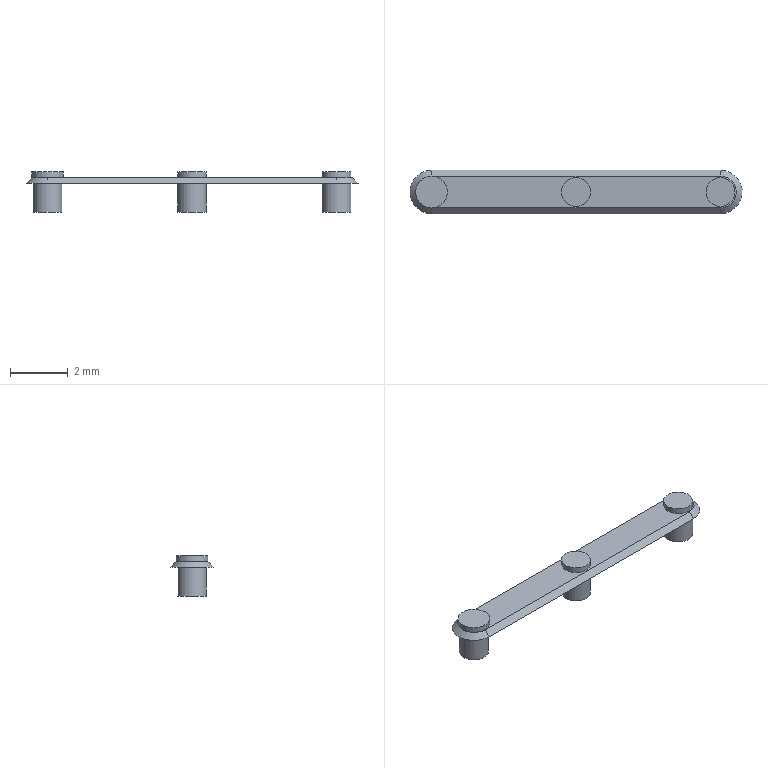Part | NX | features DATUM_CSYS 4, EXTRUDE 3, SKETCH 3, CHAMFER 1 | 7 solids | 24 faces | box 11.5 x 1.5 x 1.4 mm | volume 5.728 mm3 | plane 16 | cylinder 6 | cone 2 | commonest cylinder face diameters 1 x5 1.1 x1
STEP:
#1=CARTESIAN_POINT('',(0.5,0.,1.));
#2=VERTEX_POINT('',#1);
#3=CARTESIAN_POINT('',(0.,0.,1.));
#4=DIRECTION('',(0.,0.,1.));
#5=DIRECTION('',(1.,0.,0.));
#6=AXIS2_PLACEMENT_3D('',#3,#4,#5);
#7=CIRCLE('',#6,0.5);
#8=EDGE_CURVE('',#2,#2,#7,.T.);
#9=ORIENTED_EDGE('',*,*,#8,.F.);
#10=EDGE_LOOP('',(#9));
#11=FACE_BOUND('',#10,.T.);
#12=CARTESIAN_POINT('',(0.5,0.,0.));
#13=VERTEX_POINT('',#12);
#14=CARTESIAN_POINT('',(0.,0.,0.));
#15=DIRECTION('',(0.,0.,1.));
#16=DIRECTION('',(1.,0.,0.));
#17=AXIS2_PLACEMENT_3D('',#14,#15,#16);
#18=CIRCLE('',#17,0.5);
#19=EDGE_CURVE('',#13,#13,#18,.T.);
#20=ORIENTED_EDGE('',*,*,#19,.T.);
#21=EDGE_LOOP('',(#20));
#22=FACE_BOUND('',#21,.T.);
#23=CARTESIAN_POINT('',(0.,0.,1.));
#24=DIRECTION('',(0.,0.,-1.));
#25=DIRECTION('',(-1.,0.,0.));
#26=AXIS2_PLACEMENT_3D('',#23,#24,#25);
#27=CYLINDRICAL_SURFACE('',#26,0.5);
#28=ADVANCED_FACE('',(#11,#22),#27,.T.);
#29=ORIENTED_EDGE('',*,*,#8,.T.);
#30=EDGE_LOOP('',(#29));
#31=FACE_BOUND('',#30,.T.);
#32=CARTESIAN_POINT('',(0.,0.,1.));
#33=DIRECTION('',(0.,0.,1.));
#34=DIRECTION('',(1.,0.,0.));
#35=AXIS2_PLACEMENT_3D('',#32,#33,#34);
#36=PLANE('',#35);
#37=ADVANCED_FACE('',(#31),#36,.T.);
#38=ORIENTED_EDGE('',*,*,#19,.F.);
#39=EDGE_LOOP('',(#38));
#40=FACE_BOUND('',#39,.T.);
#41=CARTESIAN_POINT('',(0.,0.,0.));
#42=DIRECTION('',(0.,0.,1.));
#43=DIRECTION('',(1.,0.,0.));
#44=AXIS2_PLACEMENT_3D('',#41,#42,#43);
#45=PLANE('',#44);
#46=ADVANCED_FACE('',(#40),#45,.F.);
#47=CLOSED_SHELL('',(#28,#37,#46));
#48=MANIFOLD_SOLID_BREP('',#47);
#49=CARTESIAN_POINT('',(5.5,0.,1.));
#50=VERTEX_POINT('',#49);
#51=CARTESIAN_POINT('',(5.,0.,1.));
#52=DIRECTION('',(0.,0.,1.));
#53=DIRECTION('',(1.,0.,0.));
#54=AXIS2_PLACEMENT_3D('',#51,#52,#53);
#55=CIRCLE('',#54,0.5);
#56=EDGE_CURVE('',#50,#50,#55,.T.);
#57=ORIENTED_EDGE('',*,*,#56,.F.);
#58=EDGE_LOOP('',(#57));
#59=FACE_BOUND('',#58,.T.);
#60=CARTESIAN_POINT('',(5.5,0.,0.));
#61=VERTEX_POINT('',#60);
#62=CARTESIAN_POINT('',(5.,0.,0.));
#63=DIRECTION('',(0.,0.,1.));
#64=DIRECTION('',(1.,0.,0.));
#65=AXIS2_PLACEMENT_3D('',#62,#63,#64);
#66=CIRCLE('',#65,0.5);
#67=EDGE_CURVE('',#61,#61,#66,.T.);
#68=ORIENTED_EDGE('',*,*,#67,.T.);
#69=EDGE_LOOP('',(#68));
#70=FACE_BOUND('',#69,.T.);
#71=CARTESIAN_POINT('',(5.,0.,1.));
#72=DIRECTION('',(0.,0.,-1.));
#73=DIRECTION('',(-1.,0.,0.));
#74=AXIS2_PLACEMENT_3D('',#71,#72,#73);
#75=CYLINDRICAL_SURFACE('',#74,0.5);
#76=ADVANCED_FACE('',(#59,#70),#75,.T.);
#77=ORIENTED_EDGE('',*,*,#56,.T.);
#78=EDGE_LOOP('',(#77));
#79=FACE_BOUND('',#78,.T.);
#80=CARTESIAN_POINT('',(5.,0.,1.));
#81=DIRECTION('',(0.,0.,1.));
#82=DIRECTION('',(1.,0.,0.));
#83=AXIS2_PLACEMENT_3D('',#80,#81,#82);
#84=PLANE('',#83);
#85=ADVANCED_FACE('',(#79),#84,.T.);
#86=ORIENTED_EDGE('',*,*,#67,.F.);
#87=EDGE_LOOP('',(#86));
#88=FACE_BOUND('',#87,.T.);
#89=CARTESIAN_POINT('',(5.,0.,0.));
#90=DIRECTION('',(0.,0.,1.));
#91=DIRECTION('',(1.,0.,0.));
#92=AXIS2_PLACEMENT_3D('',#89,#90,#91);
#93=PLANE('',#92);
#94=ADVANCED_FACE('',(#88),#93,.F.);
#95=CLOSED_SHELL('',(#76,#85,#94));
#96=MANIFOLD_SOLID_BREP('',#95);
#97=CARTESIAN_POINT('',(10.5,0.,1.4));
#98=VERTEX_POINT('',#97);
#99=CARTESIAN_POINT('',(10.,0.,1.4));
#100=DIRECTION('',(0.,0.,1.));
#101=DIRECTION('',(1.,0.,0.));
#102=AXIS2_PLACEMENT_3D('',#99,#100,#101);
#103=CIRCLE('',#102,0.5);
#104=EDGE_CURVE('',#98,#98,#103,.T.);
#105=ORIENTED_EDGE('',*,*,#104,.F.);
#106=EDGE_LOOP('',(#105));
#107=FACE_BOUND('',#106,.T.);
#108=CARTESIAN_POINT('',(10.5,0.,1.2));
#109=VERTEX_POINT('',#108);
#110=CARTESIAN_POINT('',(10.,0.,1.2));
#111=DIRECTION('',(0.,0.,1.));
#112=DIRECTION('',(1.,0.,0.));
#113=AXIS2_PLACEMENT_3D('',#110,#111,#112);
#114=CIRCLE('',#113,0.5);
#115=EDGE_CURVE('',#109,#109,#114,.T.);
#116=ORIENTED_EDGE('',*,*,#115,.T.);
#117=EDGE_LOOP('',(#116));
#118=FACE_BOUND('',#117,.T.);
#119=CARTESIAN_POINT('',(10.,0.,1.4));
#120=DIRECTION('',(0.,0.,-1.));
#121=DIRECTION('',(-1.,0.,0.));
#122=AXIS2_PLACEMENT_3D('',#119,#120,#121);
#123=CYLINDRICAL_SURFACE('',#122,0.5);
#124=ADVANCED_FACE('',(#107,#118),#123,.T.);
#125=ORIENTED_EDGE('',*,*,#104,.T.);
#126=EDGE_LOOP('',(#125));
#127=FACE_BOUND('',#126,.T.);
#128=CARTESIAN_POINT('',(10.,0.,1.4));
#129=DIRECTION('',(0.,0.,1.));
#130=DIRECTION('',(1.,0.,0.));
#131=AXIS2_PLACEMENT_3D('',#128,#129,#130);
#132=PLANE('',#131);
#133=ADVANCED_FACE('',(#127),#132,.T.);
#134=ORIENTED_EDGE('',*,*,#115,.F.);
#135=EDGE_LOOP('',(#134));
#136=FACE_BOUND('',#135,.T.);
#137=CARTESIAN_POINT('',(10.,0.,1.2));
#138=DIRECTION('',(0.,0.,1.));
#139=DIRECTION('',(1.,0.,0.));
#140=AXIS2_PLACEMENT_3D('',#137,#138,#139);
#141=PLANE('',#140);
#142=ADVANCED_FACE('',(#136),#141,.F.);
#143=CLOSED_SHELL('',(#124,#133,#142));
#144=MANIFOLD_SOLID_BREP('',#143);
#145=CARTESIAN_POINT('',(0.55,0.,1.4));
#146=VERTEX_POINT('',#145);
#147=CARTESIAN_POINT('',(0.,0.,1.4));
#148=DIRECTION('',(0.,0.,1.));
#149=DIRECTION('',(1.,0.,0.));
#150=AXIS2_PLACEMENT_3D('',#147,#148,#149);
#151=CIRCLE('',#150,0.55);
#152=EDGE_CURVE('',#146,#146,#151,.T.);
#153=ORIENTED_EDGE('',*,*,#152,.F.);
#154=EDGE_LOOP('',(#153));
#155=FACE_BOUND('',#154,.T.);
#156=CARTESIAN_POINT('',(0.55,0.,1.2));
#157=VERTEX_POINT('',#156);
#158=CARTESIAN_POINT('',(0.,0.,1.2));
#159=DIRECTION('',(0.,0.,1.));
#160=DIRECTION('',(1.,0.,0.));
#161=AXIS2_PLACEMENT_3D('',#158,#159,#160);
#162=CIRCLE('',#161,0.55);
#163=EDGE_CURVE('',#157,#157,#162,.T.);
#164=ORIENTED_EDGE('',*,*,#163,.T.);
#165=EDGE_LOOP('',(#164));
#166=FACE_BOUND('',#165,.T.);
#167=CARTESIAN_POINT('',(0.,0.,1.4));
#168=DIRECTION('',(0.,0.,-1.));
#169=DIRECTION('',(-1.,0.,0.));
#170=AXIS2_PLACEMENT_3D('',#167,#168,#169);
#171=CYLINDRICAL_SURFACE('',#170,0.55);
#172=ADVANCED_FACE('',(#155,#166),#171,.T.);
#173=ORIENTED_EDGE('',*,*,#152,.T.);
#174=EDGE_LOOP('',(#173));
#175=FACE_BOUND('',#174,.T.);
#176=CARTESIAN_POINT('',(0.,0.,1.4));
#177=DIRECTION('',(0.,0.,1.));
#178=DIRECTION('',(1.,0.,0.));
#179=AXIS2_PLACEMENT_3D('',#176,#177,#178);
#180=PLANE('',#179);
#181=ADVANCED_FACE('',(#175),#180,.T.);
#182=ORIENTED_EDGE('',*,*,#163,.F.);
#183=EDGE_LOOP('',(#182));
#184=FACE_BOUND('',#183,.T.);
#185=CARTESIAN_POINT('',(0.,0.,1.2));
#186=DIRECTION('',(0.,0.,1.));
#187=DIRECTION('',(1.,0.,0.));
#188=AXIS2_PLACEMENT_3D('',#185,#186,#187);
#189=PLANE('',#188);
#190=ADVANCED_FACE('',(#184),#189,.F.);
#191=CLOSED_SHELL('',(#172,#181,#190));
#192=MANIFOLD_SOLID_BREP('',#191);
#193=CARTESIAN_POINT('',(10.,0.55,1.2));
#194=VERTEX_POINT('',#193);
#195=CARTESIAN_POINT('',(0.,0.55,1.2));
#196=VERTEX_POINT('',#195);
#197=CARTESIAN_POINT('',(0.,0.55,1.2));
#198=DIRECTION('',(-1.,0.,0.));
#199=VECTOR('',#198,1000.);
#200=LINE('',#197,#199);
#201=EDGE_CURVE('',#194,#196,#200,.T.);
#202=ORIENTED_EDGE('',*,*,#201,.T.);
#203=CARTESIAN_POINT('',(0.,-0.55,1.2));
#204=VERTEX_POINT('',#203);
#205=CARTESIAN_POINT('',(0.,0.,1.2));
#206=DIRECTION('',(0.,0.,1.));
#207=DIRECTION('',(1.,0.,0.));
#208=AXIS2_PLACEMENT_3D('',#205,#206,#207);
#209=CIRCLE('',#208,0.55);
#210=EDGE_CURVE('',#196,#204,#209,.T.);
#211=ORIENTED_EDGE('',*,*,#210,.T.);
#212=CARTESIAN_POINT('',(10.,-0.55,1.2));
#213=VERTEX_POINT('',#212);
#214=CARTESIAN_POINT('',(10.,-0.55,1.2));
#215=DIRECTION('',(1.,0.,0.));
#216=VECTOR('',#215,1000.);
#217=LINE('',#214,#216);
#218=EDGE_CURVE('',#204,#213,#217,.T.);
#219=ORIENTED_EDGE('',*,*,#218,.T.);
#220=CARTESIAN_POINT('',(10.,0.,1.2));
#221=DIRECTION('',(0.,0.,1.));
#222=DIRECTION('',(1.,0.,0.));
#223=AXIS2_PLACEMENT_3D('',#220,#221,#222);
#224=CIRCLE('',#223,0.55);
#225=EDGE_CURVE('',#213,#194,#224,.T.);
#226=ORIENTED_EDGE('',*,*,#225,.T.);
#227=EDGE_LOOP('',(#202,#211,#219,#226));
#228=FACE_BOUND('',#227,.T.);
#229=CARTESIAN_POINT('',(0.,0.,1.2));
#230=DIRECTION('',(0.,0.,1.));
#231=DIRECTION('',(1.,0.,0.));
#232=AXIS2_PLACEMENT_3D('',#229,#230,#231);
#233=PLANE('',#232);
#234=ADVANCED_FACE('',(#228),#233,.T.);
#235=CARTESIAN_POINT('',(0.,0.75,1.));
#236=VERTEX_POINT('',#235);
#237=CARTESIAN_POINT('',(0.,-0.75,1.));
#238=VERTEX_POINT('',#237);
#239=CARTESIAN_POINT('',(0.,0.,1.));
#240=DIRECTION('',(0.,0.,1.));
#241=DIRECTION('',(1.,0.,0.));
#242=AXIS2_PLACEMENT_3D('',#239,#240,#241);
#243=CIRCLE('',#242,0.75);
#244=EDGE_CURVE('',#236,#238,#243,.T.);
#245=ORIENTED_EDGE('',*,*,#244,.F.);
#246=CARTESIAN_POINT('',(10.,0.75,1.));
#247=VERTEX_POINT('',#246);
#248=CARTESIAN_POINT('',(10.,0.75,1.));
#249=DIRECTION('',(-1.,0.,0.));
#250=VECTOR('',#249,1000.);
#251=LINE('',#248,#250);
#252=EDGE_CURVE('',#247,#236,#251,.T.);
#253=ORIENTED_EDGE('',*,*,#252,.F.);
#254=CARTESIAN_POINT('',(10.,-0.75,1.));
#255=VERTEX_POINT('',#254);
#256=CARTESIAN_POINT('',(10.,0.,1.));
#257=DIRECTION('',(0.,0.,1.));
#258=DIRECTION('',(1.,0.,0.));
#259=AXIS2_PLACEMENT_3D('',#256,#257,#258);
#260=CIRCLE('',#259,0.75);
#261=EDGE_CURVE('',#255,#247,#260,.T.);
#262=ORIENTED_EDGE('',*,*,#261,.F.);
#263=CARTESIAN_POINT('',(0.,-0.75,1.));
#264=DIRECTION('',(1.,0.,0.));
#265=VECTOR('',#264,1000.);
#266=LINE('',#263,#265);
#267=EDGE_CURVE('',#238,#255,#266,.T.);
#268=ORIENTED_EDGE('',*,*,#267,.F.);
#269=EDGE_LOOP('',(#245,#253,#262,#268));
#270=FACE_BOUND('',#269,.T.);
#271=CARTESIAN_POINT('',(0.,0.,1.));
#272=DIRECTION('',(0.,0.,1.));
#273=DIRECTION('',(1.,0.,0.));
#274=AXIS2_PLACEMENT_3D('',#271,#272,#273);
#275=PLANE('',#274);
#276=ADVANCED_FACE('',(#270),#275,.F.);
#277=CARTESIAN_POINT('',(10.,-0.75,1.));
#278=DIRECTION('',(0.,0.7071,0.7071));
#279=VECTOR('',#278,1000.);
#280=LINE('',#277,#279);
#281=EDGE_CURVE('',#255,#213,#280,.T.);
#282=ORIENTED_EDGE('',*,*,#281,.F.);
#283=ORIENTED_EDGE('',*,*,#261,.T.);
#284=CARTESIAN_POINT('',(10.,0.55,1.2));
#285=DIRECTION('',(0.,0.7071,-0.7071));
#286=VECTOR('',#285,1000.);
#287=LINE('',#284,#286);
#288=EDGE_CURVE('',#194,#247,#287,.T.);
#289=ORIENTED_EDGE('',*,*,#288,.F.);
#290=ORIENTED_EDGE('',*,*,#225,.F.);
#291=EDGE_LOOP('',(#282,#283,#289,#290));
#292=FACE_BOUND('',#291,.T.);
#293=CARTESIAN_POINT('',(10.,0.,1.2));
#294=DIRECTION('',(0.,0.,-1.));
#295=DIRECTION('',(-1.,0.,0.));
#296=AXIS2_PLACEMENT_3D('',#293,#294,#295);
#297=CONICAL_SURFACE('',#296,0.55,0.7854);
#298=ADVANCED_FACE('',(#292),#297,.T.);
#299=ORIENTED_EDGE('',*,*,#288,.T.);
#300=ORIENTED_EDGE('',*,*,#252,.T.);
#301=CARTESIAN_POINT('',(0.,0.55,1.2));
#302=DIRECTION('',(0.,0.7071,-0.7071));
#303=VECTOR('',#302,1000.);
#304=LINE('',#301,#303);
#305=EDGE_CURVE('',#196,#236,#304,.T.);
#306=ORIENTED_EDGE('',*,*,#305,.F.);
#307=ORIENTED_EDGE('',*,*,#201,.F.);
#308=EDGE_LOOP('',(#299,#300,#306,#307));
#309=FACE_BOUND('',#308,.T.);
#310=CARTESIAN_POINT('',(0.,0.55,1.2));
#311=DIRECTION('',(0.,0.7071,0.7071));
#312=DIRECTION('',(1.,0.,0.));
#313=AXIS2_PLACEMENT_3D('',#310,#311,#312);
#314=PLANE('',#313);
#315=ADVANCED_FACE('',(#309),#314,.T.);
#316=ORIENTED_EDGE('',*,*,#281,.T.);
#317=ORIENTED_EDGE('',*,*,#218,.F.);
#318=CARTESIAN_POINT('',(0.,-0.75,1.));
#319=DIRECTION('',(0.,0.7071,0.7071));
#320=VECTOR('',#319,1000.);
#321=LINE('',#318,#320);
#322=EDGE_CURVE('',#238,#204,#321,.T.);
#323=ORIENTED_EDGE('',*,*,#322,.F.);
#324=ORIENTED_EDGE('',*,*,#267,.T.);
#325=EDGE_LOOP('',(#316,#317,#323,#324));
#326=FACE_BOUND('',#325,.T.);
#327=CARTESIAN_POINT('',(0.,-0.55,1.2));
#328=DIRECTION('',(0.,-0.7071,0.7071));
#329=DIRECTION('',(-1.,0.,0.));
#330=AXIS2_PLACEMENT_3D('',#327,#328,#329);
#331=PLANE('',#330);
#332=ADVANCED_FACE('',(#326),#331,.T.);
#333=ORIENTED_EDGE('',*,*,#305,.T.);
#334=ORIENTED_EDGE('',*,*,#244,.T.);
#335=ORIENTED_EDGE('',*,*,#322,.T.);
#336=ORIENTED_EDGE('',*,*,#210,.F.);
#337=EDGE_LOOP('',(#333,#334,#335,#336));
#338=FACE_BOUND('',#337,.T.);
#339=CARTESIAN_POINT('',(0.,0.,1.2));
#340=DIRECTION('',(0.,0.,-1.));
#341=DIRECTION('',(-1.,0.,0.));
#342=AXIS2_PLACEMENT_3D('',#339,#340,#341);
#343=CONICAL_SURFACE('',#342,0.55,0.7854);
#344=ADVANCED_FACE('',(#338),#343,.T.);
#345=CLOSED_SHELL('',(#234,#276,#298,#315,#332,#344));
#346=MANIFOLD_SOLID_BREP('',#345);
#347=CARTESIAN_POINT('',(5.5,0.,1.4));
#348=VERTEX_POINT('',#347);
#349=CARTESIAN_POINT('',(5.,0.,1.4));
#350=DIRECTION('',(0.,0.,1.));
#351=DIRECTION('',(1.,0.,0.));
#352=AXIS2_PLACEMENT_3D('',#349,#350,#351);
#353=CIRCLE('',#352,0.5);
#354=EDGE_CURVE('',#348,#348,#353,.T.);
#355=ORIENTED_EDGE('',*,*,#354,.F.);
#356=EDGE_LOOP('',(#355));
#357=FACE_BOUND('',#356,.T.);
#358=CARTESIAN_POINT('',(5.5,0.,1.2));
#359=VERTEX_POINT('',#358);
#360=CARTESIAN_POINT('',(5.,0.,1.2));
#361=DIRECTION('',(0.,0.,1.));
#362=DIRECTION('',(1.,0.,0.));
#363=AXIS2_PLACEMENT_3D('',#360,#361,#362);
#364=CIRCLE('',#363,0.5);
#365=EDGE_CURVE('',#359,#359,#364,.T.);
#366=ORIENTED_EDGE('',*,*,#365,.T.);
#367=EDGE_LOOP('',(#366));
#368=FACE_BOUND('',#367,.T.);
#369=CARTESIAN_POINT('',(5.,0.,1.4));
#370=DIRECTION('',(0.,0.,-1.));
#371=DIRECTION('',(-1.,0.,0.));
#372=AXIS2_PLACEMENT_3D('',#369,#370,#371);
#373=CYLINDRICAL_SURFACE('',#372,0.5);
#374=ADVANCED_FACE('',(#357,#368),#373,.T.);
#375=ORIENTED_EDGE('',*,*,#354,.T.);
#376=EDGE_LOOP('',(#375));
#377=FACE_BOUND('',#376,.T.);
#378=CARTESIAN_POINT('',(5.,0.,1.4));
#379=DIRECTION('',(0.,0.,1.));
#380=DIRECTION('',(1.,0.,0.));
#381=AXIS2_PLACEMENT_3D('',#378,#379,#380);
#382=PLANE('',#381);
#383=ADVANCED_FACE('',(#377),#382,.T.);
#384=ORIENTED_EDGE('',*,*,#365,.F.);
#385=EDGE_LOOP('',(#384));
#386=FACE_BOUND('',#385,.T.);
#387=CARTESIAN_POINT('',(5.,0.,1.2));
#388=DIRECTION('',(0.,0.,1.));
#389=DIRECTION('',(1.,0.,0.));
#390=AXIS2_PLACEMENT_3D('',#387,#388,#389);
#391=PLANE('',#390);
#392=ADVANCED_FACE('',(#386),#391,.F.);
#393=CLOSED_SHELL('',(#374,#383,#392));
#394=MANIFOLD_SOLID_BREP('',#393);
#395=CARTESIAN_POINT('',(10.5,0.,1.));
#396=VERTEX_POINT('',#395);
#397=CARTESIAN_POINT('',(10.,0.,1.));
#398=DIRECTION('',(0.,0.,1.));
#399=DIRECTION('',(1.,0.,0.));
#400=AXIS2_PLACEMENT_3D('',#397,#398,#399);
#401=CIRCLE('',#400,0.5);
#402=EDGE_CURVE('',#396,#396,#401,.T.);
#403=ORIENTED_EDGE('',*,*,#402,.F.);
#404=EDGE_LOOP('',(#403));
#405=FACE_BOUND('',#404,.T.);
#406=CARTESIAN_POINT('',(10.5,0.,0.));
#407=VERTEX_POINT('',#406);
#408=CARTESIAN_POINT('',(10.,0.,0.));
#409=DIRECTION('',(0.,0.,1.));
#410=DIRECTION('',(1.,0.,0.));
#411=AXIS2_PLACEMENT_3D('',#408,#409,#410);
#412=CIRCLE('',#411,0.5);
#413=EDGE_CURVE('',#407,#407,#412,.T.);
#414=ORIENTED_EDGE('',*,*,#413,.T.);
#415=EDGE_LOOP('',(#414));
#416=FACE_BOUND('',#415,.T.);
#417=CARTESIAN_POINT('',(10.,0.,1.));
#418=DIRECTION('',(0.,0.,-1.));
#419=DIRECTION('',(-1.,0.,0.));
#420=AXIS2_PLACEMENT_3D('',#417,#418,#419);
#421=CYLINDRICAL_SURFACE('',#420,0.5);
#422=ADVANCED_FACE('',(#405,#416),#421,.T.);
#423=ORIENTED_EDGE('',*,*,#402,.T.);
#424=EDGE_LOOP('',(#423));
#425=FACE_BOUND('',#424,.T.);
#426=CARTESIAN_POINT('',(10.,0.,1.));
#427=DIRECTION('',(0.,0.,1.));
#428=DIRECTION('',(1.,0.,0.));
#429=AXIS2_PLACEMENT_3D('',#426,#427,#428);
#430=PLANE('',#429);
#431=ADVANCED_FACE('',(#425),#430,.T.);
#432=ORIENTED_EDGE('',*,*,#413,.F.);
#433=EDGE_LOOP('',(#432));
#434=FACE_BOUND('',#433,.T.);
#435=CARTESIAN_POINT('',(10.,0.,0.));
#436=DIRECTION('',(0.,0.,1.));
#437=DIRECTION('',(1.,0.,0.));
#438=AXIS2_PLACEMENT_3D('',#435,#436,#437);
#439=PLANE('',#438);
#440=ADVANCED_FACE('',(#434),#439,.F.);
#441=CLOSED_SHELL('',(#422,#431,#440));
#442=MANIFOLD_SOLID_BREP('',#441);
#443=(LENGTH_UNIT()NAMED_UNIT(*)SI_UNIT(.MILLI.,.METRE.));
#444=UNCERTAINTY_MEASURE_WITH_UNIT(LENGTH_MEASURE(0.00001),#443,'','');
#445=(NAMED_UNIT(*)PLANE_ANGLE_UNIT()SI_UNIT($,.RADIAN.));
#446=(NAMED_UNIT(*)SI_UNIT($,.STERADIAN.)SOLID_ANGLE_UNIT());
#447=(GEOMETRIC_REPRESENTATION_CONTEXT(3)GLOBAL_UNCERTAINTY_ASSIGNED_CONTEXT((#444))GLOBAL_UNIT_ASSIGNED_CONTEXT((#443,#445,#446))REPRESENTATION_CONTEXT('',''));
#448=ADVANCED_BREP_SHAPE_REPRESENTATION('',(#48,#96,#144,#192,#346,#394,#442),#447);